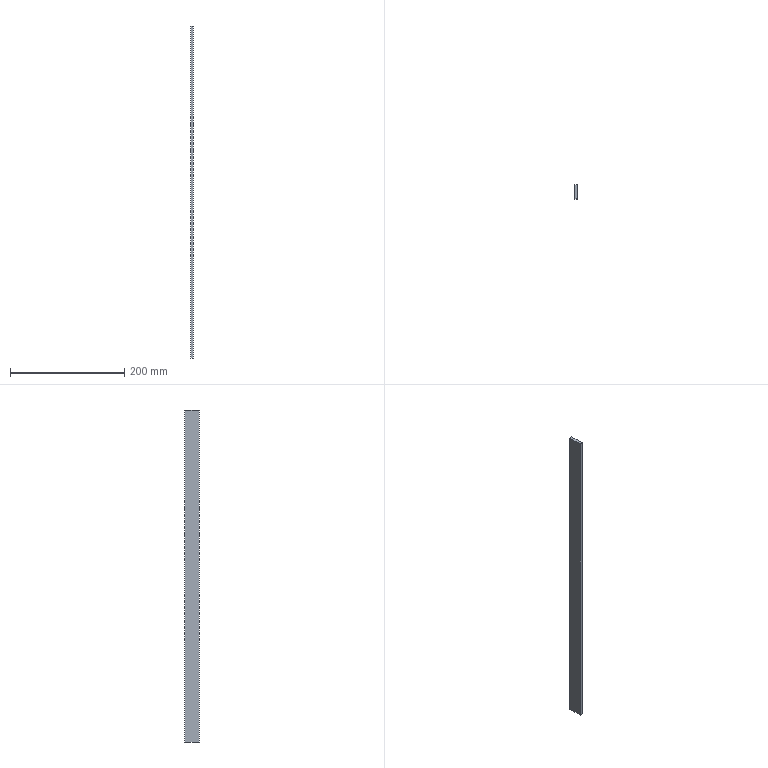Part | SolidWorks | features Extrusion 1 | 1 solid | 6 faces | box 5 x 25 x 580 mm | volume 72500 mm3 | plane 6
STEP:
#1=CARTESIAN_POINT('',(0.,25.,0.));
#2=VERTEX_POINT('',#1);
#3=CARTESIAN_POINT('',(0.,0.,0.));
#4=VERTEX_POINT('',#3);
#5=CARTESIAN_POINT('',(0.,0.,0.));
#6=DIRECTION('',(0.,-1.,0.));
#7=VECTOR('',#6,1000.);
#8=LINE('',#5,#7);
#9=EDGE_CURVE('',#2,#4,#8,.T.);
#10=ORIENTED_EDGE('',*,*,#9,.T.);
#11=CARTESIAN_POINT('',(0.,0.,580.));
#12=VERTEX_POINT('',#11);
#13=CARTESIAN_POINT('',(0.,0.,580.));
#14=DIRECTION('',(0.,0.,-1.));
#15=VECTOR('',#14,1000.);
#16=LINE('',#13,#15);
#17=EDGE_CURVE('',#12,#4,#16,.T.);
#18=ORIENTED_EDGE('',*,*,#17,.F.);
#19=CARTESIAN_POINT('',(0.,25.,580.));
#20=VERTEX_POINT('',#19);
#21=CARTESIAN_POINT('',(0.,0.,580.));
#22=DIRECTION('',(0.,-1.,0.));
#23=VECTOR('',#22,1000.);
#24=LINE('',#21,#23);
#25=EDGE_CURVE('',#20,#12,#24,.T.);
#26=ORIENTED_EDGE('',*,*,#25,.F.);
#27=CARTESIAN_POINT('',(0.,25.,580.));
#28=DIRECTION('',(0.,0.,-1.));
#29=VECTOR('',#28,1000.);
#30=LINE('',#27,#29);
#31=EDGE_CURVE('',#20,#2,#30,.T.);
#32=ORIENTED_EDGE('',*,*,#31,.T.);
#33=EDGE_LOOP('',(#10,#18,#26,#32));
#34=FACE_OUTER_BOUND('',#33,.T.);
#35=CARTESIAN_POINT('',(0.,0.,580.));
#36=DIRECTION('',(1.,0.,0.));
#37=DIRECTION('',(0.,0.,-1.));
#38=AXIS2_PLACEMENT_3D('',#35,#36,#37);
#39=PLANE('',#38);
#40=ADVANCED_FACE('',(#34),#39,.F.);
#41=CARTESIAN_POINT('',(5.,0.,0.));
#42=VERTEX_POINT('',#41);
#43=CARTESIAN_POINT('',(0.,0.,0.));
#44=DIRECTION('',(1.,0.,0.));
#45=VECTOR('',#44,1000.);
#46=LINE('',#43,#45);
#47=EDGE_CURVE('',#4,#42,#46,.T.);
#48=ORIENTED_EDGE('',*,*,#47,.T.);
#49=CARTESIAN_POINT('',(5.,0.,580.));
#50=VERTEX_POINT('',#49);
#51=CARTESIAN_POINT('',(5.,0.,580.));
#52=DIRECTION('',(0.,0.,-1.));
#53=VECTOR('',#52,1000.);
#54=LINE('',#51,#53);
#55=EDGE_CURVE('',#50,#42,#54,.T.);
#56=ORIENTED_EDGE('',*,*,#55,.F.);
#57=CARTESIAN_POINT('',(0.,0.,580.));
#58=DIRECTION('',(1.,0.,0.));
#59=VECTOR('',#58,1000.);
#60=LINE('',#57,#59);
#61=EDGE_CURVE('',#12,#50,#60,.T.);
#62=ORIENTED_EDGE('',*,*,#61,.F.);
#63=ORIENTED_EDGE('',*,*,#17,.T.);
#64=EDGE_LOOP('',(#48,#56,#62,#63));
#65=FACE_OUTER_BOUND('',#64,.T.);
#66=CARTESIAN_POINT('',(0.,0.,580.));
#67=DIRECTION('',(0.,1.,0.));
#68=DIRECTION('',(0.,0.,1.));
#69=AXIS2_PLACEMENT_3D('',#66,#67,#68);
#70=PLANE('',#69);
#71=ADVANCED_FACE('',(#65),#70,.F.);
#72=CARTESIAN_POINT('',(5.,25.,0.));
#73=VERTEX_POINT('',#72);
#74=CARTESIAN_POINT('',(5.,0.,0.));
#75=DIRECTION('',(0.,1.,0.));
#76=VECTOR('',#75,1000.);
#77=LINE('',#74,#76);
#78=EDGE_CURVE('',#42,#73,#77,.T.);
#79=ORIENTED_EDGE('',*,*,#78,.T.);
#80=CARTESIAN_POINT('',(5.,25.,580.));
#81=VERTEX_POINT('',#80);
#82=CARTESIAN_POINT('',(5.,25.,580.));
#83=DIRECTION('',(0.,0.,-1.));
#84=VECTOR('',#83,1000.);
#85=LINE('',#82,#84);
#86=EDGE_CURVE('',#81,#73,#85,.T.);
#87=ORIENTED_EDGE('',*,*,#86,.F.);
#88=CARTESIAN_POINT('',(5.,0.,580.));
#89=DIRECTION('',(0.,1.,0.));
#90=VECTOR('',#89,1000.);
#91=LINE('',#88,#90);
#92=EDGE_CURVE('',#50,#81,#91,.T.);
#93=ORIENTED_EDGE('',*,*,#92,.F.);
#94=ORIENTED_EDGE('',*,*,#55,.T.);
#95=EDGE_LOOP('',(#79,#87,#93,#94));
#96=FACE_OUTER_BOUND('',#95,.T.);
#97=CARTESIAN_POINT('',(5.,0.,580.));
#98=DIRECTION('',(-1.,0.,0.));
#99=DIRECTION('',(0.,-1.,0.));
#100=AXIS2_PLACEMENT_3D('',#97,#98,#99);
#101=PLANE('',#100);
#102=ADVANCED_FACE('',(#96),#101,.F.);
#103=CARTESIAN_POINT('',(0.,25.,0.));
#104=DIRECTION('',(-1.,0.,0.));
#105=VECTOR('',#104,1000.);
#106=LINE('',#103,#105);
#107=EDGE_CURVE('',#73,#2,#106,.T.);
#108=ORIENTED_EDGE('',*,*,#107,.T.);
#109=ORIENTED_EDGE('',*,*,#31,.F.);
#110=CARTESIAN_POINT('',(0.,25.,580.));
#111=DIRECTION('',(-1.,0.,0.));
#112=VECTOR('',#111,1000.);
#113=LINE('',#110,#112);
#114=EDGE_CURVE('',#81,#20,#113,.T.);
#115=ORIENTED_EDGE('',*,*,#114,.F.);
#116=ORIENTED_EDGE('',*,*,#86,.T.);
#117=EDGE_LOOP('',(#108,#109,#115,#116));
#118=FACE_OUTER_BOUND('',#117,.T.);
#119=CARTESIAN_POINT('',(0.,25.,580.));
#120=DIRECTION('',(0.,-1.,0.));
#121=DIRECTION('',(0.,0.,-1.));
#122=AXIS2_PLACEMENT_3D('',#119,#120,#121);
#123=PLANE('',#122);
#124=ADVANCED_FACE('',(#118),#123,.F.);
#125=ORIENTED_EDGE('',*,*,#25,.T.);
#126=ORIENTED_EDGE('',*,*,#61,.T.);
#127=ORIENTED_EDGE('',*,*,#92,.T.);
#128=ORIENTED_EDGE('',*,*,#114,.T.);
#129=EDGE_LOOP('',(#125,#126,#127,#128));
#130=FACE_OUTER_BOUND('',#129,.T.);
#131=CARTESIAN_POINT('',(0.,0.,580.));
#132=DIRECTION('',(0.,0.,-1.));
#133=DIRECTION('',(-1.,0.,0.));
#134=AXIS2_PLACEMENT_3D('',#131,#132,#133);
#135=PLANE('',#134);
#136=ADVANCED_FACE('',(#130),#135,.F.);
#137=ORIENTED_EDGE('',*,*,#9,.F.);
#138=ORIENTED_EDGE('',*,*,#107,.F.);
#139=ORIENTED_EDGE('',*,*,#78,.F.);
#140=ORIENTED_EDGE('',*,*,#47,.F.);
#141=EDGE_LOOP('',(#137,#138,#139,#140));
#142=FACE_OUTER_BOUND('',#141,.T.);
#143=CARTESIAN_POINT('',(0.,0.,0.));
#144=DIRECTION('',(0.,0.,-1.));
#145=DIRECTION('',(-1.,0.,0.));
#146=AXIS2_PLACEMENT_3D('',#143,#144,#145);
#147=PLANE('',#146);
#148=ADVANCED_FACE('',(#142),#147,.T.);
#149=CLOSED_SHELL('',(#40,#71,#102,#124,#136,#148));
#150=MANIFOLD_SOLID_BREP('',#149);
#151=CARTESIAN_POINT('',(0.,0.,0.));
#152=DIRECTION('',(0.,0.,1.));
#153=DIRECTION('',(1.,0.,0.));
#154=AXIS2_PLACEMENT_3D('',#151,#152,#153);
#155=(LENGTH_UNIT()NAMED_UNIT(*)SI_UNIT(.MILLI.,.METRE.));
#156=UNCERTAINTY_MEASURE_WITH_UNIT(LENGTH_MEASURE(0.00001),#155,'','');
#157=(NAMED_UNIT(*)PLANE_ANGLE_UNIT()SI_UNIT($,.RADIAN.));
#158=(NAMED_UNIT(*)SI_UNIT($,.STERADIAN.)SOLID_ANGLE_UNIT());
#159=(GEOMETRIC_REPRESENTATION_CONTEXT(3)GLOBAL_UNCERTAINTY_ASSIGNED_CONTEXT((#156))GLOBAL_UNIT_ASSIGNED_CONTEXT((#155,#157,#158))REPRESENTATION_CONTEXT('',''));
#160=ADVANCED_BREP_SHAPE_REPRESENTATION('',(#150,#154),#159);